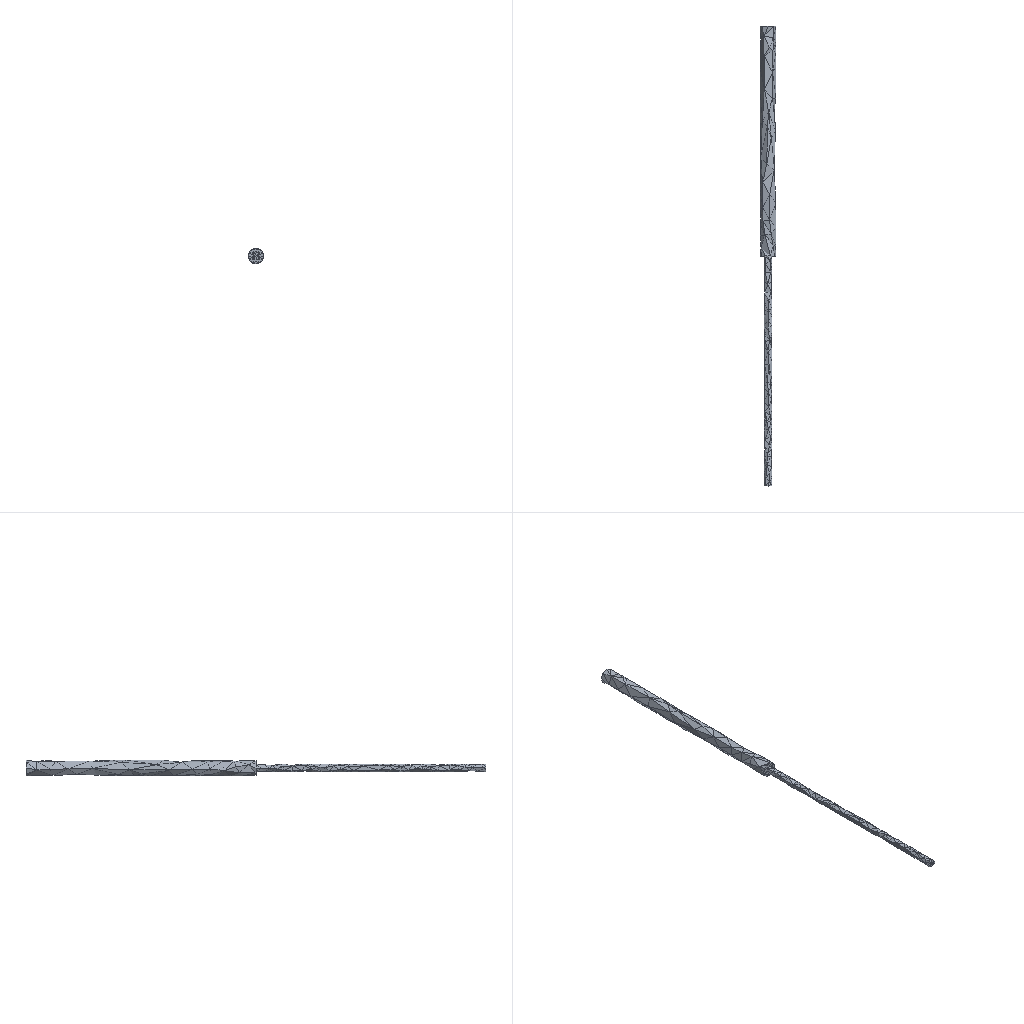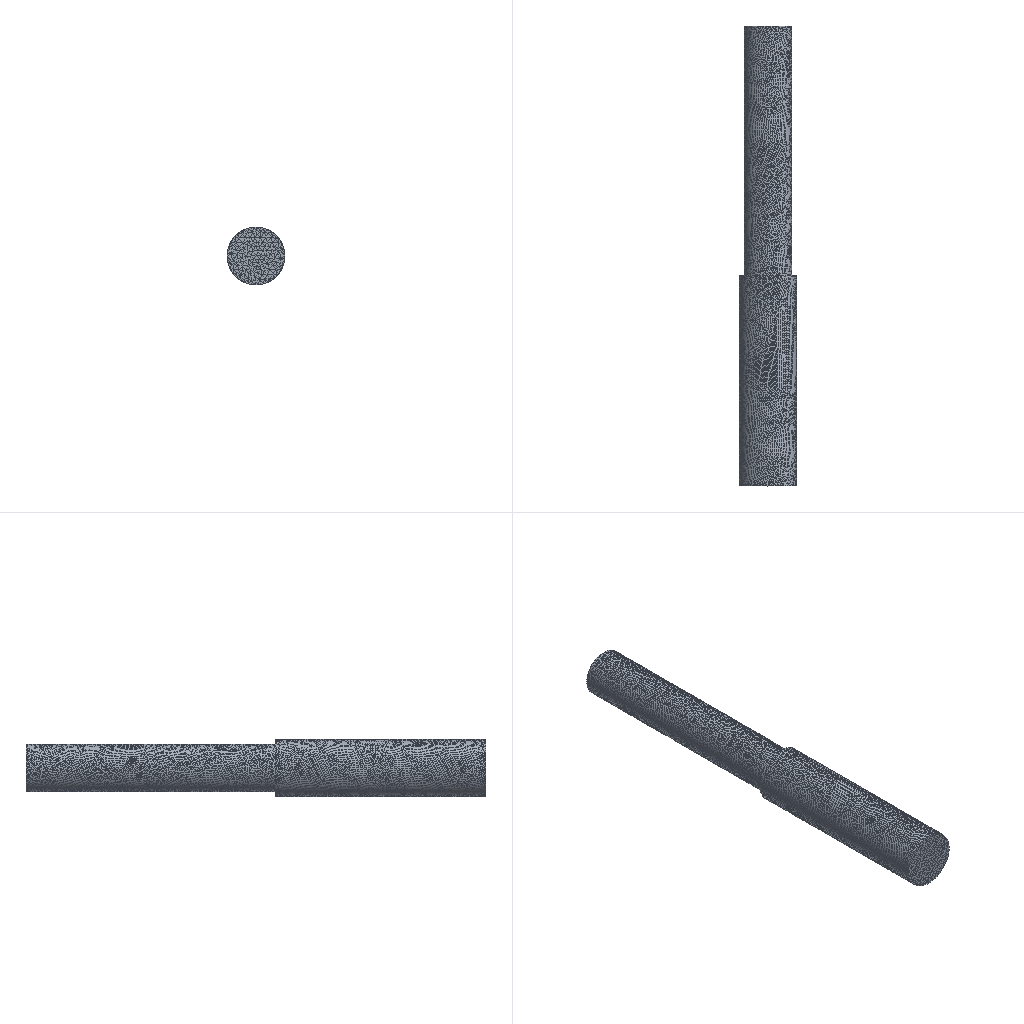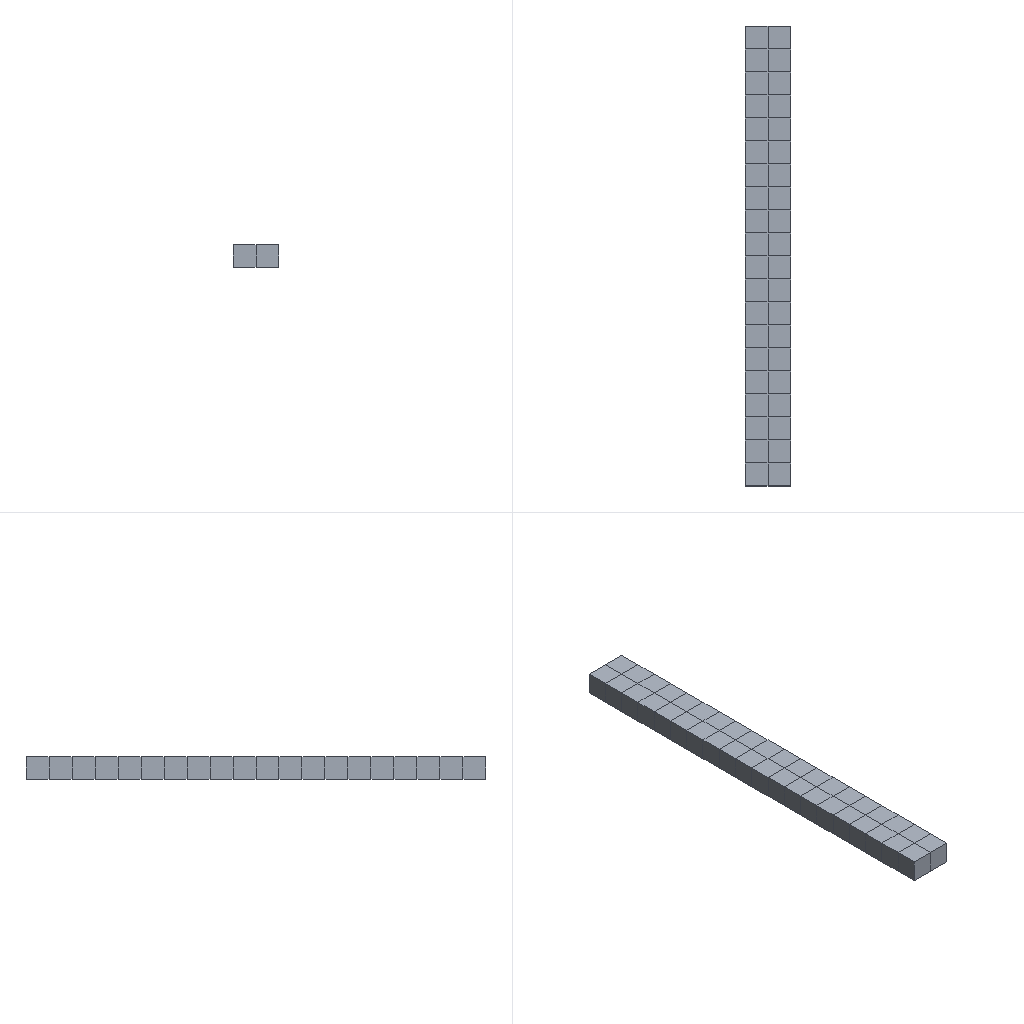Simulation study | ansys workbench
Set-up summary:
category,name,step,type,value,unit,region
solver,ansys_mapdl
solver,version,,,22.1
solver,version,,,22.1
solver,version,,,22.1
units,MPA,,stated
analysis,deck1,,static,static
load_step,requested,,,1
analysis,nlgeom,,,False
mesh,nodes,,,122160
mesh,elements,,,70482
element_type,ANSYS 187 (type 1),,solid,70267
element_type,ANSYS 177 (type 2),,contact,76
element_type,ANSYS 170 (type 3),,target,0
element_type,ANSYS 177 (type 4),,contact,76
element_type,ANSYS 170 (type 5),,target,0
element_type,ANSYS 177 (type 6),,contact,63
element_type,ANSYS 170 (type 7),,target,0
load,load commands in deck,,count,9
bc,support commands in deck,,count,1
named_set,_FIXEDSU,,component
analysis,deck2,,static,static
load_step,requested,,,1
analysis,nlgeom,,,False
mesh,nodes,,,393
mesh,elements,,,41
element_type,ANSYS 186 (type 1),,solid,40
element_type,ANSYS 156 (type 2),,surface,1
load,load commands in deck,,count,3
bc,support commands in deck,,count,1
named_set,_FIXEDSU,,component
analysis,deck3,,static,static
load_step,requested,,,1
analysis,nlgeom,,,False
mesh,nodes,,,1252
mesh,elements,,,582
element_type,ANSYS 187 (type 1),,solid,552
element_type,ANSYS 154 (type 2),,surface,6
element_type,ANSYS 154 (type 3),,surface,6
element_type,ANSYS 154 (type 4),,surface,18
load,load commands in deck,,count,9
bc,support commands in deck,,count,3
named_set,_DISPZEROUX,,component
named_set,_DISPZEROUZ,,component
named_set,_FIXEDSU,,component
material,1,,in results
material,1,,in results
material,1,,in results
check,setup vs results,,match,results also hold 0 node(s) and 3 element(s) the deck makes with ['EN']; those were not compared; 3 node(s) the solver created internally for pilot nodes (ansys有限元题目分析22/ansys有限元题目分析/1_files/dp0/SYS-1/MECH/solve.out) are in the results only
check,setup vs results,,match,1 surface effect element(s) are not in the reader's mesh and were not compared
check,setup vs results,,match,30 surface effect element(s) are not in the reader's mesh and were not compared
Results summary:
result,analysis,,,static
result,last_loadstep,,,1
result,primary field,,,displacement
result,reaction total,1,FX,0.000138,N
result,reaction total,1,FY,0.00039,N
result,reaction total,1,FZ,0.00015,N
result,mass,,,0.07123,"NMM: mm, ton, N, s, mV, mA, degC"
result,analysis,,,static
result,last_loadstep,,,1
result,primary field,,,displacement
result,reaction total,1,FX,-10000,N
result,reaction total,1,FY,0.0,N
result,reaction total,1,FZ,0.0,N
result,mass,,,0.03925,"NMM: mm, ton, N, s, mV, mA, degC"
result,analysis,,,static
result,last_loadstep,,,1
result,primary field,,,displacement
result,reaction total,1,FX,-0.0,N
result,reaction total,1,FY,-900000,N
result,reaction total,1,FZ,0.0,N
result,mass,,,0.000905,"NMM: mm, ton, N, s, mV, mA, degC"